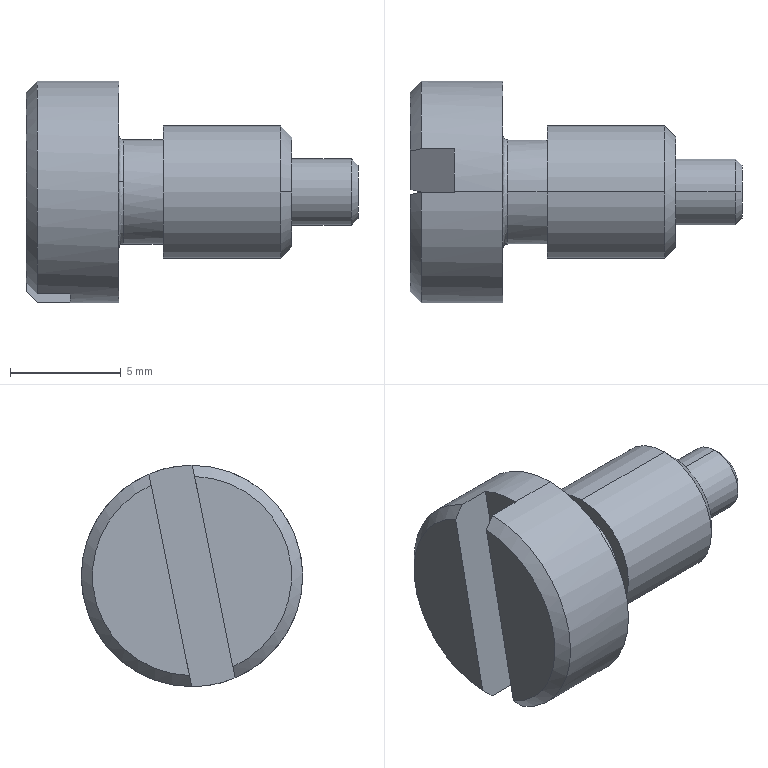Part | SolidWorks | features BaseBody 1 | 1 solid | 25 faces | box 15 x 10 x 10 mm | volume 504.228 mm3 | plane 9 | cylinder 8 | cone 6 | spline 2 | commonest cylinder face diameters 3 x2 4.7 x2 6 x2 10 x2
STEP:
#1=CARTESIAN_POINT('',(-32.901,8.92,2.5));
#2=VERTEX_POINT('',#1);
#3=CARTESIAN_POINT('',(-32.901,8.92,12.5));
#4=VERTEX_POINT('',#3);
#5=CARTESIAN_POINT('',(-32.901,8.92,7.5));
#6=DIRECTION('',(1.,0.,0.));
#7=DIRECTION('',(0.,0.,1.));
#8=AXIS2_PLACEMENT_3D('',#5,#6,#7);
#9=CIRCLE('',#8,5.);
#10=EDGE_CURVE('',#2,#4,#9,.T.);
#11=ORIENTED_EDGE('',*,*,#10,.F.);
#12=CARTESIAN_POINT('',(-35.101,8.92,2.5));
#13=VERTEX_POINT('',#12);
#14=CARTESIAN_POINT('',(-32.901,8.92,2.5));
#15=DIRECTION('',(-1.,0.,0.));
#16=VECTOR('',#15,1000.);
#17=LINE('',#14,#16);
#18=EDGE_CURVE('',#2,#13,#17,.T.);
#19=ORIENTED_EDGE('',*,*,#18,.T.);
#20=CARTESIAN_POINT('',(-35.101,8.937,2.5));
#21=VERTEX_POINT('',#20);
#22=CARTESIAN_POINT('',(-35.101,8.92,7.5));
#23=DIRECTION('',(1.,0.,0.));
#24=DIRECTION('',(0.,0.,1.));
#25=AXIS2_PLACEMENT_3D('',#22,#23,#24);
#26=CIRCLE('',#25,5.);
#27=EDGE_CURVE('',#13,#21,#26,.T.);
#28=ORIENTED_EDGE('',*,*,#27,.T.);
#29=CARTESIAN_POINT('',(-36.601,8.937,2.5));
#30=VERTEX_POINT('',#29);
#31=CARTESIAN_POINT('',(-36.101,8.937,2.5));
#32=DIRECTION('',(-1.,0.,0.));
#33=VECTOR('',#32,1000.);
#34=LINE('',#31,#33);
#35=EDGE_CURVE('',#21,#30,#34,.T.);
#36=ORIENTED_EDGE('',*,*,#35,.T.);
#37=CARTESIAN_POINT('',(-36.601,10.864,12.107));
#38=VERTEX_POINT('',#37);
#39=CARTESIAN_POINT('',(-36.601,8.92,7.5));
#40=DIRECTION('',(1.,0.,0.));
#41=DIRECTION('',(0.,0.,1.));
#42=AXIS2_PLACEMENT_3D('',#39,#40,#41);
#43=CIRCLE('',#42,5.);
#44=EDGE_CURVE('',#30,#38,#43,.T.);
#45=ORIENTED_EDGE('',*,*,#44,.T.);
#46=CARTESIAN_POINT('',(-35.101,10.864,12.107));
#47=VERTEX_POINT('',#46);
#48=CARTESIAN_POINT('',(-36.101,10.864,12.107));
#49=DIRECTION('',(1.,0.,0.));
#50=VECTOR('',#49,1000.);
#51=LINE('',#48,#50);
#52=EDGE_CURVE('',#38,#47,#51,.T.);
#53=ORIENTED_EDGE('',*,*,#52,.T.);
#54=CARTESIAN_POINT('',(-35.101,8.92,12.5));
#55=VERTEX_POINT('',#54);
#56=CARTESIAN_POINT('',(-35.101,8.92,7.5));
#57=DIRECTION('',(1.,0.,0.));
#58=DIRECTION('',(0.,0.,1.));
#59=AXIS2_PLACEMENT_3D('',#56,#57,#58);
#60=CIRCLE('',#59,5.);
#61=EDGE_CURVE('',#47,#55,#60,.T.);
#62=ORIENTED_EDGE('',*,*,#61,.T.);
#63=CARTESIAN_POINT('',(-32.901,8.92,12.5));
#64=DIRECTION('',(-1.,0.,0.));
#65=VECTOR('',#64,1000.);
#66=LINE('',#63,#65);
#67=EDGE_CURVE('',#4,#55,#66,.T.);
#68=ORIENTED_EDGE('',*,*,#67,.F.);
#69=EDGE_LOOP('',(#11,#19,#28,#36,#45,#53,#62,#68));
#70=FACE_OUTER_BOUND('',#69,.T.);
#71=CARTESIAN_POINT('',(-32.901,8.92,7.5));
#72=DIRECTION('',(-1.,0.,0.));
#73=DIRECTION('',(0.,0.,1.));
#74=AXIS2_PLACEMENT_3D('',#71,#72,#73);
#75=CYLINDRICAL_SURFACE('',#74,5.);
#76=ADVANCED_FACE('',(#70),#75,.T.);
#77=CARTESIAN_POINT('',(-30.901,8.92,9.85));
#78=VERTEX_POINT('',#77);
#79=CARTESIAN_POINT('',(-30.901,8.92,5.15));
#80=VERTEX_POINT('',#79);
#81=CARTESIAN_POINT('',(-30.901,8.92,7.5));
#82=DIRECTION('',(-1.,0.,0.));
#83=DIRECTION('',(0.,0.,1.));
#84=AXIS2_PLACEMENT_3D('',#81,#82,#83);
#85=CIRCLE('',#84,2.35);
#86=EDGE_CURVE('',#78,#80,#85,.T.);
#87=ORIENTED_EDGE('',*,*,#86,.T.);
#88=CARTESIAN_POINT('',(-32.701,8.92,5.15));
#89=VERTEX_POINT('',#88);
#90=CARTESIAN_POINT('',(-30.901,8.92,5.15));
#91=DIRECTION('',(-1.,0.,0.));
#92=VECTOR('',#91,1000.);
#93=LINE('',#90,#92);
#94=EDGE_CURVE('',#80,#89,#93,.T.);
#95=ORIENTED_EDGE('',*,*,#94,.T.);
#96=CARTESIAN_POINT('',(-32.701,11.224,7.038));
#97=VERTEX_POINT('',#96);
#98=CARTESIAN_POINT('',(-32.701,8.92,7.5));
#99=DIRECTION('',(1.,0.,0.000000002));
#100=DIRECTION('',(0.,0.9805,-0.1967));
#101=AXIS2_PLACEMENT_3D('',#98,#99,#100);
#102=CIRCLE('',#101,2.35);
#103=EDGE_CURVE('',#89,#97,#102,.T.);
#104=ORIENTED_EDGE('',*,*,#103,.T.);
#105=CARTESIAN_POINT('',(-32.701,8.92,9.85));
#106=VERTEX_POINT('',#105);
#107=CARTESIAN_POINT('',(-32.701,8.92,7.5));
#108=DIRECTION('',(1.,-0.000000001,-0.000000003));
#109=DIRECTION('',(0.,-0.9805,0.1967));
#110=AXIS2_PLACEMENT_3D('',#107,#108,#109);
#111=CIRCLE('',#110,2.35);
#112=EDGE_CURVE('',#97,#106,#111,.T.);
#113=ORIENTED_EDGE('',*,*,#112,.T.);
#114=CARTESIAN_POINT('',(-30.901,8.92,9.85));
#115=DIRECTION('',(-1.,0.,0.));
#116=VECTOR('',#115,1000.);
#117=LINE('',#114,#116);
#118=EDGE_CURVE('',#78,#106,#117,.T.);
#119=ORIENTED_EDGE('',*,*,#118,.F.);
#120=EDGE_LOOP('',(#87,#95,#104,#113,#119));
#121=FACE_OUTER_BOUND('',#120,.T.);
#122=CARTESIAN_POINT('',(-30.901,8.92,7.5));
#123=DIRECTION('',(-1.,0.,0.));
#124=DIRECTION('',(0.,0.,1.));
#125=AXIS2_PLACEMENT_3D('',#122,#123,#124);
#126=CYLINDRICAL_SURFACE('',#125,2.35);
#127=ADVANCED_FACE('',(#121),#126,.T.);
#128=CARTESIAN_POINT('',(-25.601,11.92,7.5));
#129=VERTEX_POINT('',#128);
#130=CARTESIAN_POINT('',(-25.601,8.92,4.5));
#131=VERTEX_POINT('',#130);
#132=CARTESIAN_POINT('',(-25.601,8.92,7.5));
#133=DIRECTION('',(-1.,0.,0.));
#134=DIRECTION('',(0.,0.,1.));
#135=AXIS2_PLACEMENT_3D('',#132,#133,#134);
#136=CIRCLE('',#135,3.);
#137=EDGE_CURVE('',#129,#131,#136,.T.);
#138=ORIENTED_EDGE('',*,*,#137,.T.);
#139=CARTESIAN_POINT('',(-30.901,8.92,4.5));
#140=VERTEX_POINT('',#139);
#141=CARTESIAN_POINT('',(-25.601,8.92,4.5));
#142=DIRECTION('',(-1.,0.,0.));
#143=VECTOR('',#142,1000.);
#144=LINE('',#141,#143);
#145=EDGE_CURVE('',#131,#140,#144,.T.);
#146=ORIENTED_EDGE('',*,*,#145,.T.);
#147=CARTESIAN_POINT('',(-30.901,8.92,10.5));
#148=VERTEX_POINT('',#147);
#149=CARTESIAN_POINT('',(-30.901,8.92,7.5));
#150=DIRECTION('',(1.,0.,0.));
#151=DIRECTION('',(0.,0.,1.));
#152=AXIS2_PLACEMENT_3D('',#149,#150,#151);
#153=CIRCLE('',#152,3.);
#154=EDGE_CURVE('',#140,#148,#153,.T.);
#155=ORIENTED_EDGE('',*,*,#154,.T.);
#156=CARTESIAN_POINT('',(-25.601,8.92,10.5));
#157=VERTEX_POINT('',#156);
#158=CARTESIAN_POINT('',(-25.601,8.92,10.5));
#159=DIRECTION('',(-1.,0.,0.));
#160=VECTOR('',#159,1000.);
#161=LINE('',#158,#160);
#162=EDGE_CURVE('',#157,#148,#161,.T.);
#163=ORIENTED_EDGE('',*,*,#162,.F.);
#164=CARTESIAN_POINT('',(-25.601,8.92,7.5));
#165=DIRECTION('',(-1.,0.,0.));
#166=DIRECTION('',(0.,0.,1.));
#167=AXIS2_PLACEMENT_3D('',#164,#165,#166);
#168=CIRCLE('',#167,3.);
#169=EDGE_CURVE('',#157,#129,#168,.T.);
#170=ORIENTED_EDGE('',*,*,#169,.T.);
#171=EDGE_LOOP('',(#138,#146,#155,#163,#170));
#172=FACE_OUTER_BOUND('',#171,.T.);
#173=CARTESIAN_POINT('',(-25.601,8.92,7.5));
#174=DIRECTION('',(-1.,0.,0.));
#175=DIRECTION('',(0.,0.,1.));
#176=AXIS2_PLACEMENT_3D('',#173,#174,#175);
#177=CYLINDRICAL_SURFACE('',#176,3.);
#178=ADVANCED_FACE('',(#172),#177,.T.);
#179=CARTESIAN_POINT('',(-25.101,6.42,7.5));
#180=VERTEX_POINT('',#179);
#181=CARTESIAN_POINT('',(-25.101,11.42,7.5));
#182=VERTEX_POINT('',#181);
#183=CARTESIAN_POINT('',(-25.101,8.92,7.5));
#184=DIRECTION('',(-1.,0.,0.));
#185=DIRECTION('',(0.,-1.,0.));
#186=AXIS2_PLACEMENT_3D('',#183,#184,#185);
#187=CIRCLE('',#186,2.5);
#188=EDGE_CURVE('',#180,#182,#187,.T.);
#189=ORIENTED_EDGE('',*,*,#188,.T.);
#190=CARTESIAN_POINT('',(-25.601,11.92,7.5));
#191=DIRECTION('',(-0.7071,0.7071,0.));
#192=VECTOR('',#191,1000.);
#193=LINE('',#190,#192);
#194=EDGE_CURVE('',#182,#129,#193,.T.);
#195=ORIENTED_EDGE('',*,*,#194,.T.);
#196=ORIENTED_EDGE('',*,*,#169,.F.);
#197=CARTESIAN_POINT('',(-25.601,5.92,7.5));
#198=VERTEX_POINT('',#197);
#199=CARTESIAN_POINT('',(-25.601,8.92,7.5));
#200=DIRECTION('',(-1.,0.,0.));
#201=DIRECTION('',(0.,0.,1.));
#202=AXIS2_PLACEMENT_3D('',#199,#200,#201);
#203=CIRCLE('',#202,3.);
#204=EDGE_CURVE('',#198,#157,#203,.T.);
#205=ORIENTED_EDGE('',*,*,#204,.F.);
#206=CARTESIAN_POINT('',(-25.601,5.92,7.5));
#207=DIRECTION('',(-0.7071,-0.7071,0.));
#208=VECTOR('',#207,1000.);
#209=LINE('',#206,#208);
#210=EDGE_CURVE('',#180,#198,#209,.T.);
#211=ORIENTED_EDGE('',*,*,#210,.F.);
#212=EDGE_LOOP('',(#189,#195,#196,#205,#211));
#213=FACE_OUTER_BOUND('',#212,.T.);
#214=CARTESIAN_POINT('',(-25.601,8.92,7.5));
#215=DIRECTION('',(-1.,0.,0.));
#216=DIRECTION('',(0.,-1.,0.));
#217=AXIS2_PLACEMENT_3D('',#214,#215,#216);
#218=CONICAL_SURFACE('',#217,3.,0.7854);
#219=ADVANCED_FACE('',(#213),#218,.T.);
#220=CARTESIAN_POINT('',(-22.401,8.92,9.));
#221=VERTEX_POINT('',#220);
#222=CARTESIAN_POINT('',(-22.401,8.92,6.));
#223=VERTEX_POINT('',#222);
#224=CARTESIAN_POINT('',(-22.401,8.92,7.5));
#225=DIRECTION('',(-1.,0.,0.));
#226=DIRECTION('',(0.,0.,1.));
#227=AXIS2_PLACEMENT_3D('',#224,#225,#226);
#228=CIRCLE('',#227,1.5);
#229=EDGE_CURVE('',#221,#223,#228,.T.);
#230=ORIENTED_EDGE('',*,*,#229,.T.);
#231=CARTESIAN_POINT('',(-25.101,8.92,6.));
#232=VERTEX_POINT('',#231);
#233=CARTESIAN_POINT('',(-22.401,8.92,6.));
#234=DIRECTION('',(-1.,0.,0.));
#235=VECTOR('',#234,1000.);
#236=LINE('',#233,#235);
#237=EDGE_CURVE('',#223,#232,#236,.T.);
#238=ORIENTED_EDGE('',*,*,#237,.T.);
#239=CARTESIAN_POINT('',(-25.101,8.92,9.));
#240=VERTEX_POINT('',#239);
#241=CARTESIAN_POINT('',(-25.101,8.92,7.5));
#242=DIRECTION('',(-1.,0.,0.));
#243=DIRECTION('',(0.,0.,1.));
#244=AXIS2_PLACEMENT_3D('',#241,#242,#243);
#245=CIRCLE('',#244,1.5);
#246=EDGE_CURVE('',#240,#232,#245,.T.);
#247=ORIENTED_EDGE('',*,*,#246,.F.);
#248=CARTESIAN_POINT('',(-22.401,8.92,9.));
#249=DIRECTION('',(-1.,0.,0.));
#250=VECTOR('',#249,1000.);
#251=LINE('',#248,#250);
#252=EDGE_CURVE('',#221,#240,#251,.T.);
#253=ORIENTED_EDGE('',*,*,#252,.F.);
#254=EDGE_LOOP('',(#230,#238,#247,#253));
#255=FACE_OUTER_BOUND('',#254,.T.);
#256=CARTESIAN_POINT('',(-22.401,8.92,7.5));
#257=DIRECTION('',(-1.,0.,0.));
#258=DIRECTION('',(0.,0.,1.));
#259=AXIS2_PLACEMENT_3D('',#256,#257,#258);
#260=CYLINDRICAL_SURFACE('',#259,1.5);
#261=ADVANCED_FACE('',(#255),#260,.T.);
#262=CARTESIAN_POINT('',(-22.101,8.92,8.7));
#263=VERTEX_POINT('',#262);
#264=CARTESIAN_POINT('',(-22.101,8.92,6.3));
#265=VERTEX_POINT('',#264);
#266=CARTESIAN_POINT('',(-22.101,8.92,7.5));
#267=DIRECTION('',(-1.,0.,0.));
#268=DIRECTION('',(0.,0.,1.));
#269=AXIS2_PLACEMENT_3D('',#266,#267,#268);
#270=CIRCLE('',#269,1.2);
#271=EDGE_CURVE('',#263,#265,#270,.T.);
#272=ORIENTED_EDGE('',*,*,#271,.T.);
#273=CARTESIAN_POINT('',(-22.401,8.92,6.));
#274=DIRECTION('',(-0.7071,0.,-0.7071));
#275=VECTOR('',#274,1000.);
#276=LINE('',#273,#275);
#277=EDGE_CURVE('',#265,#223,#276,.T.);
#278=ORIENTED_EDGE('',*,*,#277,.T.);
#279=ORIENTED_EDGE('',*,*,#229,.F.);
#280=CARTESIAN_POINT('',(-22.401,8.92,9.));
#281=DIRECTION('',(-0.7071,0.,0.7071));
#282=VECTOR('',#281,1000.);
#283=LINE('',#280,#282);
#284=EDGE_CURVE('',#263,#221,#283,.T.);
#285=ORIENTED_EDGE('',*,*,#284,.F.);
#286=EDGE_LOOP('',(#272,#278,#279,#285));
#287=FACE_OUTER_BOUND('',#286,.T.);
#288=CARTESIAN_POINT('',(-22.401,8.92,7.5));
#289=DIRECTION('',(-1.,0.,0.));
#290=DIRECTION('',(0.,0.,1.));
#291=AXIS2_PLACEMENT_3D('',#288,#289,#290);
#292=CONICAL_SURFACE('',#291,1.5,0.7854);
#293=ADVANCED_FACE('',(#287),#292,.T.);
#294=CARTESIAN_POINT('',(-32.901,6.42,8.002));
#295=VERTEX_POINT('',#294);
#296=CARTESIAN_POINT('',(-32.901,11.42,6.998));
#297=VERTEX_POINT('',#296);
#298=CARTESIAN_POINT('',(-32.901,6.42,8.002));
#299=CARTESIAN_POINT('',(-32.901,6.452,8.161));
#300=CARTESIAN_POINT('',(-32.901,6.52,8.39));
#301=CARTESIAN_POINT('',(-32.901,6.638,8.643));
#302=CARTESIAN_POINT('',(-32.901,6.706,8.766));
#303=CARTESIAN_POINT('',(-32.901,6.737,8.818));
#304=CARTESIAN_POINT('',(-32.901,6.758,8.853));
#305=CARTESIAN_POINT('',(-32.901,6.768,8.868));
#306=CARTESIAN_POINT('',(-32.901,6.971,9.182));
#307=CARTESIAN_POINT('',(-32.901,7.214,9.428));
#308=CARTESIAN_POINT('',(-32.901,7.653,9.72));
#309=CARTESIAN_POINT('',(-32.901,7.883,9.842));
#310=CARTESIAN_POINT('',(-32.901,8.168,9.94));
#311=CARTESIAN_POINT('',(-32.901,8.316,9.978));
#312=CARTESIAN_POINT('',(-32.901,8.38,9.992));
#313=CARTESIAN_POINT('',(-32.901,8.423,10.001));
#314=CARTESIAN_POINT('',(-32.901,8.446,10.006));
#315=CARTESIAN_POINT('',(-32.901,8.785,10.067));
#316=CARTESIAN_POINT('',(-32.901,9.104,10.064));
#317=CARTESIAN_POINT('',(-32.901,9.58,9.968));
#318=CARTESIAN_POINT('',(-32.901,9.81,9.899));
#319=CARTESIAN_POINT('',(-32.901,10.063,9.782));
#320=CARTESIAN_POINT('',(-32.901,10.186,9.714));
#321=CARTESIAN_POINT('',(-32.901,10.238,9.683));
#322=CARTESIAN_POINT('',(-32.901,10.272,9.662));
#323=CARTESIAN_POINT('',(-32.901,10.288,9.652));
#324=CARTESIAN_POINT('',(-32.901,10.602,9.449));
#325=CARTESIAN_POINT('',(-32.901,10.847,9.206));
#326=CARTESIAN_POINT('',(-32.901,11.14,8.767));
#327=CARTESIAN_POINT('',(-32.901,11.261,8.537));
#328=CARTESIAN_POINT('',(-32.901,11.36,8.251));
#329=CARTESIAN_POINT('',(-32.901,11.398,8.104));
#330=CARTESIAN_POINT('',(-32.901,11.412,8.04));
#331=CARTESIAN_POINT('',(-32.901,11.421,7.997));
#332=CARTESIAN_POINT('',(-32.901,11.425,7.974));
#333=CARTESIAN_POINT('',(-32.901,11.487,7.635));
#334=CARTESIAN_POINT('',(-32.901,11.484,7.316));
#335=CARTESIAN_POINT('',(-32.901,11.42,6.998));
#336=B_SPLINE_CURVE_WITH_KNOTS('',3,(#298,#299,#300,#301,#302,#303,#304,#305,#306,#307,#308,#309,#310,#311,#312,#313,#314,#315,#316,#317,#318,#319,#320,#321,#322,#323,#324,#325,#326,#327,#328,#329,#330,#331,#332,#333,#334,#335),.UNSPECIFIED.,.F.,.F.,(4,1,1,1,2,2,2,1,1,1,2,2,2,1,1,1,2,2,2,1,1,1,2,2,4),(0.,0.0625,0.09375,0.1094,0.1172,0.125,0.25,0.3125,0.3438,0.3594,0.3672,0.375,0.5,0.5625,0.5938,0.6094,0.6172,0.625,0.75,0.8125,0.8437,0.8594,0.8672,0.875,1.),.UNSPECIFIED.);
#337=EDGE_CURVE('',#295,#297,#336,.T.);
#338=ORIENTED_EDGE('',*,*,#337,.T.);
#339=CARTESIAN_POINT('',(-32.901,11.42,6.998));
#340=CARTESIAN_POINT('',(-32.901,11.387,6.834));
#341=CARTESIAN_POINT('',(-32.901,11.315,6.597));
#342=CARTESIAN_POINT('',(-32.901,11.209,6.373));
#343=CARTESIAN_POINT('',(-32.901,11.131,6.227));
#344=CARTESIAN_POINT('',(-32.901,11.09,6.158));
#345=CARTESIAN_POINT('',(-32.901,10.946,5.943));
#346=CARTESIAN_POINT('',(-32.901,10.785,5.746));
#347=CARTESIAN_POINT('',(-32.901,10.565,5.548));
#348=CARTESIAN_POINT('',(-32.901,10.464,5.47));
#349=CARTESIAN_POINT('',(-32.901,10.395,5.419));
#350=CARTESIAN_POINT('',(-32.901,10.358,5.394));
#351=CARTESIAN_POINT('',(-32.901,10.185,5.28));
#352=CARTESIAN_POINT('',(-32.901,9.969,5.166));
#353=CARTESIAN_POINT('',(-32.901,9.702,5.07));
#354=CARTESIAN_POINT('',(-32.901,9.583,5.037));
#355=CARTESIAN_POINT('',(-32.901,9.504,5.017));
#356=CARTESIAN_POINT('',(-32.901,9.465,5.009));
#357=CARTESIAN_POINT('',(-32.901,9.088,4.933));
#358=CARTESIAN_POINT('',(-32.901,8.753,4.933));
#359=CARTESIAN_POINT('',(-32.901,8.251,5.033));
#360=CARTESIAN_POINT('',(-32.901,8.01,5.107));
#361=CARTESIAN_POINT('',(-32.901,7.745,5.234));
#362=CARTESIAN_POINT('',(-32.901,7.635,5.297));
#363=CARTESIAN_POINT('',(-32.901,7.562,5.341));
#364=CARTESIAN_POINT('',(-32.901,7.525,5.365));
#365=CARTESIAN_POINT('',(-32.901,7.354,5.48));
#366=CARTESIAN_POINT('',(-32.901,7.166,5.636));
#367=CARTESIAN_POINT('',(-32.901,6.975,5.847));
#368=CARTESIAN_POINT('',(-32.901,6.9,5.943));
#369=CARTESIAN_POINT('',(-32.901,6.851,6.009));
#370=CARTESIAN_POINT('',(-32.901,6.828,6.041));
#371=CARTESIAN_POINT('',(-32.901,6.708,6.22));
#372=CARTESIAN_POINT('',(-32.901,6.587,6.444));
#373=CARTESIAN_POINT('',(-32.901,6.488,6.723));
#374=CARTESIAN_POINT('',(-32.901,6.454,6.847));
#375=CARTESIAN_POINT('',(-32.901,6.434,6.93));
#376=CARTESIAN_POINT('',(-32.901,6.425,6.973));
#377=CARTESIAN_POINT('',(-32.901,6.353,7.343));
#378=CARTESIAN_POINT('',(-32.901,6.354,7.672));
#379=CARTESIAN_POINT('',(-32.901,6.42,8.002));
#380=B_SPLINE_CURVE_WITH_KNOTS('',3,(#339,#340,#341,#342,#343,#344,#345,#346,#347,#348,#349,#350,#351,#352,#353,#354,#355,#356,#357,#358,#359,#360,#361,#362,#363,#364,#365,#366,#367,#368,#369,#370,#371,#372,#373,#374,#375,#376,#377,#378,#379),.UNSPECIFIED.,.F.,.F.,(4,1,2,2,1,1,2,2,1,1,2,2,2,1,1,2,2,1,1,2,2,1,1,2,2,4),(0.,0.0625,0.09375,0.125,0.1875,0.2187,0.2344,0.25,0.3125,0.3437,0.3594,0.375,0.5,0.5625,0.5937,0.6094,0.625,0.6875,0.7187,0.7344,0.75,0.8125,0.8437,0.8594,0.875,1.),.UNSPECIFIED.);
#381=EDGE_CURVE('',#297,#295,#380,.T.);
#382=ORIENTED_EDGE('',*,*,#381,.T.);
#383=EDGE_LOOP('',(#338,#382));
#384=FACE_BOUND('',#383,.T.);
#385=CARTESIAN_POINT('',(-32.901,8.92,7.5));
#386=DIRECTION('',(1.,0.,0.));
#387=DIRECTION('',(0.,0.,1.));
#388=AXIS2_PLACEMENT_3D('',#385,#386,#387);
#389=CIRCLE('',#388,5.);
#390=EDGE_CURVE('',#4,#2,#389,.T.);
#391=ORIENTED_EDGE('',*,*,#390,.T.);
#392=ORIENTED_EDGE('',*,*,#10,.T.);
#393=EDGE_LOOP('',(#391,#392));
#394=FACE_OUTER_BOUND('',#393,.T.);
#395=CARTESIAN_POINT('',(-32.901,8.92,7.5));
#396=DIRECTION('',(1.,0.,0.));
#397=DIRECTION('',(0.,0.,-1.));
#398=AXIS2_PLACEMENT_3D('',#395,#396,#397);
#399=PLANE('',#398);
#400=ADVANCED_FACE('',(#384,#394),#399,.T.);
#401=CARTESIAN_POINT('',(-32.701,6.616,7.962));
#402=VERTEX_POINT('',#401);
#403=CARTESIAN_POINT('',(-32.701,8.92,7.5));
#404=DIRECTION('',(1.,0.,0.000000002));
#405=DIRECTION('',(0.,0.9805,-0.1967));
#406=AXIS2_PLACEMENT_3D('',#403,#404,#405);
#407=CIRCLE('',#406,2.35);
#408=EDGE_CURVE('',#402,#89,#407,.T.);
#409=ORIENTED_EDGE('',*,*,#408,.F.);
#410=CARTESIAN_POINT('',(-32.701,6.42,8.002));
#411=DIRECTION('',(0.000000002,-0.1967,-0.9805));
#412=DIRECTION('',(0.,-0.9805,0.1967));
#413=AXIS2_PLACEMENT_3D('',#410,#411,#412);
#414=CIRCLE('',#413,0.2);
#415=EDGE_CURVE('',#295,#402,#414,.T.);
#416=ORIENTED_EDGE('',*,*,#415,.F.);
#417=ORIENTED_EDGE('',*,*,#381,.F.);
#418=CARTESIAN_POINT('',(-32.701,11.42,6.998));
#419=DIRECTION('',(-0.000000003,-0.1967,-0.9805));
#420=DIRECTION('',(0.,0.9805,-0.1967));
#421=AXIS2_PLACEMENT_3D('',#418,#419,#420);
#422=CIRCLE('',#421,0.2);
#423=EDGE_CURVE('',#97,#297,#422,.T.);
#424=ORIENTED_EDGE('',*,*,#423,.F.);
#425=ORIENTED_EDGE('',*,*,#103,.F.);
#426=EDGE_LOOP('',(#409,#416,#417,#424,#425));
#427=FACE_OUTER_BOUND('',#426,.T.);
#428=CARTESIAN_POINT('',(-32.701,11.224,7.038));
#429=CARTESIAN_POINT('',(-32.701,10.953,5.688));
#430=CARTESIAN_POINT('',(-32.701,9.807,4.925));
#431=CARTESIAN_POINT('',(-32.701,8.458,5.196));
#432=CARTESIAN_POINT('',(-32.701,7.108,5.467));
#433=CARTESIAN_POINT('',(-32.701,6.345,6.613));
#434=CARTESIAN_POINT('',(-32.701,6.616,7.962));
#435=CARTESIAN_POINT('',(-32.818,11.224,7.038));
#436=CARTESIAN_POINT('',(-32.818,10.953,5.688));
#437=CARTESIAN_POINT('',(-32.818,9.807,4.925));
#438=CARTESIAN_POINT('',(-32.818,8.458,5.196));
#439=CARTESIAN_POINT('',(-32.818,7.108,5.467));
#440=CARTESIAN_POINT('',(-32.818,6.345,6.613));
#441=CARTESIAN_POINT('',(-32.818,6.616,7.962));
#442=CARTESIAN_POINT('',(-32.901,11.305,7.021));
#443=CARTESIAN_POINT('',(-32.901,11.025,5.624));
#444=CARTESIAN_POINT('',(-32.901,9.838,4.834));
#445=CARTESIAN_POINT('',(-32.901,8.441,5.115));
#446=CARTESIAN_POINT('',(-32.901,7.044,5.395));
#447=CARTESIAN_POINT('',(-32.901,6.254,6.581));
#448=CARTESIAN_POINT('',(-32.901,6.535,7.979));
#449=CARTESIAN_POINT('',(-32.901,11.42,6.998));
#450=CARTESIAN_POINT('',(-32.901,11.126,5.534));
#451=CARTESIAN_POINT('',(-32.901,9.883,4.706));
#452=CARTESIAN_POINT('',(-32.901,8.418,5.));
#453=CARTESIAN_POINT('',(-32.901,6.954,5.294));
#454=CARTESIAN_POINT('',(-32.901,6.126,6.537));
#455=CARTESIAN_POINT('',(-32.901,6.42,8.002));
#456=(BOUNDED_SURFACE()B_SPLINE_SURFACE(3,3,((#428,#429,#430,#431,#432,#433,#434),(#435,#436,#437,#438,#439,#440,#441),(#442,#443,#444,#445,#446,#447,#448),(#449,#450,#451,#452,#453,#454,#455)),.UNSPECIFIED.,.F.,.F.,.T.)B_SPLINE_SURFACE_WITH_KNOTS((4,4),(4,3,4),(0.,1.),(0.,0.5,1.),.UNSPECIFIED.)GEOMETRIC_REPRESENTATION_ITEM()RATIONAL_B_SPLINE_SURFACE(((1.,0.8047,0.8047,1.,0.8047,0.8047,1.),(0.8047,0.6476,0.6476,0.8047,0.6476,0.6476,0.8047),(0.8047,0.6476,0.6476,0.8047,0.6476,0.6476,0.8047),(1.,0.8047,0.8047,1.,0.8047,0.8047,1.)))REPRESENTATION_ITEM('')SURFACE());
#457=ADVANCED_FACE('',(#427),#456,.F.);
#458=ORIENTED_EDGE('',*,*,#337,.F.);
#459=ORIENTED_EDGE('',*,*,#415,.T.);
#460=CARTESIAN_POINT('',(-32.701,8.92,7.5));
#461=DIRECTION('',(1.,-0.000000001,-0.000000003));
#462=DIRECTION('',(0.,-0.9805,0.1967));
#463=AXIS2_PLACEMENT_3D('',#460,#461,#462);
#464=CIRCLE('',#463,2.35);
#465=EDGE_CURVE('',#106,#402,#464,.T.);
#466=ORIENTED_EDGE('',*,*,#465,.F.);
#467=ORIENTED_EDGE('',*,*,#112,.F.);
#468=ORIENTED_EDGE('',*,*,#423,.T.);
#469=EDGE_LOOP('',(#458,#459,#466,#467,#468));
#470=FACE_OUTER_BOUND('',#469,.T.);
#471=CARTESIAN_POINT('',(-32.701,6.616,7.962));
#472=CARTESIAN_POINT('',(-32.701,6.887,9.312));
#473=CARTESIAN_POINT('',(-32.701,8.032,10.075));
#474=CARTESIAN_POINT('',(-32.701,9.382,9.804));
#475=CARTESIAN_POINT('',(-32.701,10.732,9.533));
#476=CARTESIAN_POINT('',(-32.701,11.495,8.387));
#477=CARTESIAN_POINT('',(-32.701,11.224,7.038));
#478=CARTESIAN_POINT('',(-32.818,6.616,7.962));
#479=CARTESIAN_POINT('',(-32.818,6.887,9.312));
#480=CARTESIAN_POINT('',(-32.818,8.032,10.075));
#481=CARTESIAN_POINT('',(-32.818,9.382,9.804));
#482=CARTESIAN_POINT('',(-32.818,10.732,9.533));
#483=CARTESIAN_POINT('',(-32.818,11.495,8.387));
#484=CARTESIAN_POINT('',(-32.818,11.224,7.038));
#485=CARTESIAN_POINT('',(-32.901,6.535,7.979));
#486=CARTESIAN_POINT('',(-32.901,6.815,9.376));
#487=CARTESIAN_POINT('',(-32.901,8.001,10.166));
#488=CARTESIAN_POINT('',(-32.901,9.398,9.885));
#489=CARTESIAN_POINT('',(-32.901,10.796,9.605));
#490=CARTESIAN_POINT('',(-32.901,11.585,8.419));
#491=CARTESIAN_POINT('',(-32.901,11.305,7.021));
#492=CARTESIAN_POINT('',(-32.901,6.42,8.002));
#493=CARTESIAN_POINT('',(-32.901,6.713,9.466));
#494=CARTESIAN_POINT('',(-32.901,7.957,10.294));
#495=CARTESIAN_POINT('',(-32.901,9.421,10.));
#496=CARTESIAN_POINT('',(-32.901,10.886,9.706));
#497=CARTESIAN_POINT('',(-32.901,11.714,8.463));
#498=CARTESIAN_POINT('',(-32.901,11.42,6.998));
#499=(BOUNDED_SURFACE()B_SPLINE_SURFACE(3,3,((#471,#472,#473,#474,#475,#476,#477),(#478,#479,#480,#481,#482,#483,#484),(#485,#486,#487,#488,#489,#490,#491),(#492,#493,#494,#495,#496,#497,#498)),.UNSPECIFIED.,.F.,.F.,.T.)B_SPLINE_SURFACE_WITH_KNOTS((4,4),(4,3,4),(0.,1.),(0.,0.5,1.),.UNSPECIFIED.)GEOMETRIC_REPRESENTATION_ITEM()RATIONAL_B_SPLINE_SURFACE(((1.,0.8047,0.8047,1.,0.8047,0.8047,1.),(0.8047,0.6476,0.6476,0.8047,0.6476,0.6476,0.8047),(0.8047,0.6476,0.6476,0.8047,0.6476,0.6476,0.8047),(1.,0.8047,0.8047,1.,0.8047,0.8047,1.)))REPRESENTATION_ITEM('')SURFACE());
#500=ADVANCED_FACE('',(#470),#499,.F.);
#501=ORIENTED_EDGE('',*,*,#18,.F.);
#502=ORIENTED_EDGE('',*,*,#390,.F.);
#503=ORIENTED_EDGE('',*,*,#67,.T.);
#504=CARTESIAN_POINT('',(-35.101,8.903,12.5));
#505=VERTEX_POINT('',#504);
#506=CARTESIAN_POINT('',(-35.101,8.92,7.5));
#507=DIRECTION('',(1.,0.,0.));
#508=DIRECTION('',(0.,0.,1.));
#509=AXIS2_PLACEMENT_3D('',#506,#507,#508);
#510=CIRCLE('',#509,5.);
#511=EDGE_CURVE('',#55,#505,#510,.T.);
#512=ORIENTED_EDGE('',*,*,#511,.T.);
#513=CARTESIAN_POINT('',(-36.601,8.903,12.5));
#514=VERTEX_POINT('',#513);
#515=CARTESIAN_POINT('',(-36.101,8.903,12.5));
#516=DIRECTION('',(1.,0.,0.));
#517=VECTOR('',#516,1000.);
#518=LINE('',#515,#517);
#519=EDGE_CURVE('',#514,#505,#518,.T.);
#520=ORIENTED_EDGE('',*,*,#519,.F.);
#521=CARTESIAN_POINT('',(-36.601,6.976,2.893));
#522=VERTEX_POINT('',#521);
#523=CARTESIAN_POINT('',(-36.601,8.92,7.5));
#524=DIRECTION('',(1.,0.,0.));
#525=DIRECTION('',(0.,0.,1.));
#526=AXIS2_PLACEMENT_3D('',#523,#524,#525);
#527=CIRCLE('',#526,5.);
#528=EDGE_CURVE('',#514,#522,#527,.T.);
#529=ORIENTED_EDGE('',*,*,#528,.T.);
#530=CARTESIAN_POINT('',(-35.101,6.976,2.893));
#531=VERTEX_POINT('',#530);
#532=CARTESIAN_POINT('',(-36.101,6.976,2.893));
#533=DIRECTION('',(-1.,0.,0.));
#534=VECTOR('',#533,1000.);
#535=LINE('',#532,#534);
#536=EDGE_CURVE('',#531,#522,#535,.T.);
#537=ORIENTED_EDGE('',*,*,#536,.F.);
#538=CARTESIAN_POINT('',(-35.101,8.92,7.5));
#539=DIRECTION('',(1.,0.,0.));
#540=DIRECTION('',(0.,0.,1.));
#541=AXIS2_PLACEMENT_3D('',#538,#539,#540);
#542=CIRCLE('',#541,5.);
#543=EDGE_CURVE('',#531,#13,#542,.T.);
#544=ORIENTED_EDGE('',*,*,#543,.T.);
#545=EDGE_LOOP('',(#501,#502,#503,#512,#520,#529,#537,#544));
#546=FACE_OUTER_BOUND('',#545,.T.);
#547=CARTESIAN_POINT('',(-32.901,8.92,7.5));
#548=DIRECTION('',(-1.,0.,0.));
#549=DIRECTION('',(0.,0.,1.));
#550=AXIS2_PLACEMENT_3D('',#547,#548,#549);
#551=CYLINDRICAL_SURFACE('',#550,5.);
#552=ADVANCED_FACE('',(#546),#551,.T.);
#553=ORIENTED_EDGE('',*,*,#94,.F.);
#554=CARTESIAN_POINT('',(-30.901,8.92,7.5));
#555=DIRECTION('',(-1.,0.,0.));
#556=DIRECTION('',(0.,0.,1.));
#557=AXIS2_PLACEMENT_3D('',#554,#555,#556);
#558=CIRCLE('',#557,2.35);
#559=EDGE_CURVE('',#80,#78,#558,.T.);
#560=ORIENTED_EDGE('',*,*,#559,.T.);
#561=ORIENTED_EDGE('',*,*,#118,.T.);
#562=ORIENTED_EDGE('',*,*,#465,.T.);
#563=ORIENTED_EDGE('',*,*,#408,.T.);
#564=EDGE_LOOP('',(#553,#560,#561,#562,#563));
#565=FACE_OUTER_BOUND('',#564,.T.);
#566=CARTESIAN_POINT('',(-30.901,8.92,7.5));
#567=DIRECTION('',(-1.,0.,0.));
#568=DIRECTION('',(0.,0.,1.));
#569=AXIS2_PLACEMENT_3D('',#566,#567,#568);
#570=CYLINDRICAL_SURFACE('',#569,2.35);
#571=ADVANCED_FACE('',(#565),#570,.T.);
#572=ORIENTED_EDGE('',*,*,#44,.F.);
#573=CARTESIAN_POINT('',(-37.101,9.037,3.002));
#574=VERTEX_POINT('',#573);
#575=CARTESIAN_POINT('',(-36.601,8.937,2.5));
#576=CARTESIAN_POINT('',(-36.768,8.97,2.667));
#577=CARTESIAN_POINT('',(-36.935,9.004,2.834));
#578=CARTESIAN_POINT('',(-37.101,9.037,3.002));
#579=B_SPLINE_CURVE_WITH_KNOTS('',3,(#575,#576,#577,#578),.UNSPECIFIED.,.F.,.F.,(4,4),(0.,0.0007153),.UNSPECIFIED.);
#580=EDGE_CURVE('',#30,#574,#579,.T.);
#581=ORIENTED_EDGE('',*,*,#580,.T.);
#582=CARTESIAN_POINT('',(-37.101,10.763,11.605));
#583=VERTEX_POINT('',#582);
#584=CARTESIAN_POINT('',(-37.101,8.92,7.5));
#585=DIRECTION('',(1.,0.,0.));
#586=DIRECTION('',(0.,0.,-1.));
#587=AXIS2_PLACEMENT_3D('',#584,#585,#586);
#588=CIRCLE('',#587,4.5);
#589=EDGE_CURVE('',#574,#583,#588,.T.);
#590=ORIENTED_EDGE('',*,*,#589,.T.);
#591=CARTESIAN_POINT('',(-37.101,10.763,11.605));
#592=CARTESIAN_POINT('',(-36.935,10.797,11.772));
#593=CARTESIAN_POINT('',(-36.768,10.83,11.94));
#594=CARTESIAN_POINT('',(-36.601,10.864,12.107));
#595=B_SPLINE_CURVE_WITH_KNOTS('',3,(#591,#592,#593,#594),.UNSPECIFIED.,.F.,.F.,(4,4),(0.,0.0007153),.UNSPECIFIED.);
#596=EDGE_CURVE('',#583,#38,#595,.T.);
#597=ORIENTED_EDGE('',*,*,#596,.T.);
#598=EDGE_LOOP('',(#572,#581,#590,#597));
#599=FACE_OUTER_BOUND('',#598,.T.);
#600=CARTESIAN_POINT('',(-36.601,8.92,7.5));
#601=DIRECTION('',(1.,0.,0.));
#602=DIRECTION('',(0.,0.,-1.));
#603=AXIS2_PLACEMENT_3D('',#600,#601,#602);
#604=CONICAL_SURFACE('',#603,5.,0.7854);
#605=ADVANCED_FACE('',(#599),#604,.T.);
#606=ORIENTED_EDGE('',*,*,#61,.F.);
#607=CARTESIAN_POINT('',(-35.101,8.937,2.5));
#608=DIRECTION('',(0.,0.1967,0.9805));
#609=VECTOR('',#608,1000.);
#610=LINE('',#607,#609);
#611=EDGE_CURVE('',#21,#47,#610,.T.);
#612=ORIENTED_EDGE('',*,*,#611,.F.);
#613=ORIENTED_EDGE('',*,*,#27,.F.);
#614=ORIENTED_EDGE('',*,*,#543,.F.);
#615=CARTESIAN_POINT('',(-35.101,8.903,12.5));
#616=DIRECTION('',(0.,-0.1967,-0.9805));
#617=VECTOR('',#616,1000.);
#618=LINE('',#615,#617);
#619=EDGE_CURVE('',#505,#531,#618,.T.);
#620=ORIENTED_EDGE('',*,*,#619,.F.);
#621=ORIENTED_EDGE('',*,*,#511,.F.);
#622=EDGE_LOOP('',(#606,#612,#613,#614,#620,#621));
#623=FACE_OUTER_BOUND('',#622,.T.);
#624=CARTESIAN_POINT('',(-35.101,8.92,7.5));
#625=DIRECTION('',(1.,0.,0.));
#626=DIRECTION('',(0.,0.,-1.));
#627=AXIS2_PLACEMENT_3D('',#624,#625,#626);
#628=PLANE('',#627);
#629=ADVANCED_FACE('',(#623),#628,.F.);
#630=CARTESIAN_POINT('',(-37.101,8.802,11.998));
#631=VERTEX_POINT('',#630);
#632=CARTESIAN_POINT('',(-37.101,7.076,3.395));
#633=VERTEX_POINT('',#632);
#634=CARTESIAN_POINT('',(-37.101,8.92,7.5));
#635=DIRECTION('',(1.,0.,0.));
#636=DIRECTION('',(0.,0.,-1.));
#637=AXIS2_PLACEMENT_3D('',#634,#635,#636);
#638=CIRCLE('',#637,4.5);
#639=EDGE_CURVE('',#631,#633,#638,.T.);
#640=ORIENTED_EDGE('',*,*,#639,.T.);
#641=CARTESIAN_POINT('',(-37.101,7.076,3.395));
#642=CARTESIAN_POINT('',(-36.935,7.043,3.228));
#643=CARTESIAN_POINT('',(-36.768,7.009,3.06));
#644=CARTESIAN_POINT('',(-36.601,6.976,2.893));
#645=B_SPLINE_CURVE_WITH_KNOTS('',3,(#641,#642,#643,#644),.UNSPECIFIED.,.F.,.F.,(4,4),(0.,0.0007153),.UNSPECIFIED.);
#646=EDGE_CURVE('',#633,#522,#645,.T.);
#647=ORIENTED_EDGE('',*,*,#646,.T.);
#648=ORIENTED_EDGE('',*,*,#528,.F.);
#649=CARTESIAN_POINT('',(-36.601,8.903,12.5));
#650=CARTESIAN_POINT('',(-36.768,8.87,12.333));
#651=CARTESIAN_POINT('',(-36.935,8.836,12.166));
#652=CARTESIAN_POINT('',(-37.101,8.802,11.998));
#653=B_SPLINE_CURVE_WITH_KNOTS('',3,(#649,#650,#651,#652),.UNSPECIFIED.,.F.,.F.,(4,4),(0.,0.0007153),.UNSPECIFIED.);
#654=EDGE_CURVE('',#514,#631,#653,.T.);
#655=ORIENTED_EDGE('',*,*,#654,.T.);
#656=EDGE_LOOP('',(#640,#647,#648,#655));
#657=FACE_OUTER_BOUND('',#656,.T.);
#658=CARTESIAN_POINT('',(-36.601,8.92,7.5));
#659=DIRECTION('',(1.,0.,0.));
#660=DIRECTION('',(0.,0.,-1.));
#661=AXIS2_PLACEMENT_3D('',#658,#659,#660);
#662=CONICAL_SURFACE('',#661,5.,0.7854);
#663=ADVANCED_FACE('',(#657),#662,.T.);
#664=ORIENTED_EDGE('',*,*,#86,.F.);
#665=ORIENTED_EDGE('',*,*,#559,.F.);
#666=EDGE_LOOP('',(#664,#665));
#667=FACE_BOUND('',#666,.T.);
#668=CARTESIAN_POINT('',(-30.901,8.92,7.5));
#669=DIRECTION('',(1.,0.,0.));
#670=DIRECTION('',(0.,0.,1.));
#671=AXIS2_PLACEMENT_3D('',#668,#669,#670);
#672=CIRCLE('',#671,3.);
#673=EDGE_CURVE('',#148,#140,#672,.T.);
#674=ORIENTED_EDGE('',*,*,#673,.F.);
#675=ORIENTED_EDGE('',*,*,#154,.F.);
#676=EDGE_LOOP('',(#674,#675));
#677=FACE_OUTER_BOUND('',#676,.T.);
#678=CARTESIAN_POINT('',(-30.901,8.92,7.5));
#679=DIRECTION('',(1.,0.,0.));
#680=DIRECTION('',(0.,0.,-1.));
#681=AXIS2_PLACEMENT_3D('',#678,#679,#680);
#682=PLANE('',#681);
#683=ADVANCED_FACE('',(#667,#677),#682,.F.);
#684=ORIENTED_EDGE('',*,*,#589,.F.);
#685=CARTESIAN_POINT('',(-37.101,10.763,11.605));
#686=DIRECTION('',(0.,-0.1967,-0.9805));
#687=VECTOR('',#686,1000.);
#688=LINE('',#685,#687);
#689=EDGE_CURVE('',#583,#574,#688,.T.);
#690=ORIENTED_EDGE('',*,*,#689,.F.);
#691=EDGE_LOOP('',(#684,#690));
#692=FACE_OUTER_BOUND('',#691,.T.);
#693=CARTESIAN_POINT('',(-37.101,11.229,7.303));
#694=DIRECTION('',(1.,0.,0.));
#695=DIRECTION('',(0.,0.,-1.));
#696=AXIS2_PLACEMENT_3D('',#693,#694,#695);
#697=PLANE('',#696);
#698=ADVANCED_FACE('',(#692),#697,.F.);
#699=ORIENTED_EDGE('',*,*,#519,.T.);
#700=ORIENTED_EDGE('',*,*,#619,.T.);
#701=ORIENTED_EDGE('',*,*,#536,.T.);
#702=ORIENTED_EDGE('',*,*,#646,.F.);
#703=CARTESIAN_POINT('',(-37.101,7.939,7.697));
#704=DIRECTION('',(0.,0.1967,0.9805));
#705=VECTOR('',#704,1000.);
#706=LINE('',#703,#705);
#707=EDGE_CURVE('',#633,#631,#706,.T.);
#708=ORIENTED_EDGE('',*,*,#707,.T.);
#709=ORIENTED_EDGE('',*,*,#654,.F.);
#710=EDGE_LOOP('',(#699,#700,#701,#702,#708,#709));
#711=FACE_OUTER_BOUND('',#710,.T.);
#712=CARTESIAN_POINT('',(-36.101,7.939,7.697));
#713=DIRECTION('',(0.,0.9805,-0.1967));
#714=DIRECTION('',(0.,0.1967,0.9805));
#715=AXIS2_PLACEMENT_3D('',#712,#713,#714);
#716=PLANE('',#715);
#717=ADVANCED_FACE('',(#711),#716,.T.);
#718=ORIENTED_EDGE('',*,*,#52,.F.);
#719=ORIENTED_EDGE('',*,*,#596,.F.);
#720=ORIENTED_EDGE('',*,*,#689,.T.);
#721=ORIENTED_EDGE('',*,*,#580,.F.);
#722=ORIENTED_EDGE('',*,*,#35,.F.);
#723=ORIENTED_EDGE('',*,*,#611,.T.);
#724=EDGE_LOOP('',(#718,#719,#720,#721,#722,#723));
#725=FACE_OUTER_BOUND('',#724,.T.);
#726=CARTESIAN_POINT('',(-36.101,9.9,7.303));
#727=DIRECTION('',(0.,0.9805,-0.1967));
#728=DIRECTION('',(0.,0.1967,0.9805));
#729=AXIS2_PLACEMENT_3D('',#726,#727,#728);
#730=PLANE('',#729);
#731=ADVANCED_FACE('',(#725),#730,.F.);
#732=ORIENTED_EDGE('',*,*,#639,.F.);
#733=ORIENTED_EDGE('',*,*,#707,.F.);
#734=EDGE_LOOP('',(#732,#733));
#735=FACE_OUTER_BOUND('',#734,.T.);
#736=CARTESIAN_POINT('',(-37.101,6.611,7.697));
#737=DIRECTION('',(1.,0.,0.));
#738=DIRECTION('',(0.,0.,-1.));
#739=AXIS2_PLACEMENT_3D('',#736,#737,#738);
#740=PLANE('',#739);
#741=ADVANCED_FACE('',(#735),#740,.F.);
#742=ORIENTED_EDGE('',*,*,#145,.F.);
#743=CARTESIAN_POINT('',(-25.601,8.92,7.5));
#744=DIRECTION('',(-1.,0.,0.));
#745=DIRECTION('',(0.,0.,1.));
#746=AXIS2_PLACEMENT_3D('',#743,#744,#745);
#747=CIRCLE('',#746,3.);
#748=EDGE_CURVE('',#131,#198,#747,.T.);
#749=ORIENTED_EDGE('',*,*,#748,.T.);
#750=ORIENTED_EDGE('',*,*,#204,.T.);
#751=ORIENTED_EDGE('',*,*,#162,.T.);
#752=ORIENTED_EDGE('',*,*,#673,.T.);
#753=EDGE_LOOP('',(#742,#749,#750,#751,#752));
#754=FACE_OUTER_BOUND('',#753,.T.);
#755=CARTESIAN_POINT('',(-25.601,8.92,7.5));
#756=DIRECTION('',(-1.,0.,0.));
#757=DIRECTION('',(0.,0.,1.));
#758=AXIS2_PLACEMENT_3D('',#755,#756,#757);
#759=CYLINDRICAL_SURFACE('',#758,3.);
#760=ADVANCED_FACE('',(#754),#759,.T.);
#761=ORIENTED_EDGE('',*,*,#194,.F.);
#762=CARTESIAN_POINT('',(-25.101,8.92,7.5));
#763=DIRECTION('',(-1.,0.,0.));
#764=DIRECTION('',(0.,-1.,0.));
#765=AXIS2_PLACEMENT_3D('',#762,#763,#764);
#766=CIRCLE('',#765,2.5);
#767=EDGE_CURVE('',#182,#180,#766,.T.);
#768=ORIENTED_EDGE('',*,*,#767,.T.);
#769=ORIENTED_EDGE('',*,*,#210,.T.);
#770=ORIENTED_EDGE('',*,*,#748,.F.);
#771=ORIENTED_EDGE('',*,*,#137,.F.);
#772=EDGE_LOOP('',(#761,#768,#769,#770,#771));
#773=FACE_OUTER_BOUND('',#772,.T.);
#774=CARTESIAN_POINT('',(-25.601,8.92,7.5));
#775=DIRECTION('',(-1.,0.,0.));
#776=DIRECTION('',(0.,-1.,0.));
#777=AXIS2_PLACEMENT_3D('',#774,#775,#776);
#778=CONICAL_SURFACE('',#777,3.,0.7854);
#779=ADVANCED_FACE('',(#773),#778,.T.);
#780=ORIENTED_EDGE('',*,*,#246,.T.);
#781=CARTESIAN_POINT('',(-25.101,8.92,7.5));
#782=DIRECTION('',(-1.,0.,0.));
#783=DIRECTION('',(0.,0.,1.));
#784=AXIS2_PLACEMENT_3D('',#781,#782,#783);
#785=CIRCLE('',#784,1.5);
#786=EDGE_CURVE('',#232,#240,#785,.T.);
#787=ORIENTED_EDGE('',*,*,#786,.T.);
#788=EDGE_LOOP('',(#780,#787));
#789=FACE_BOUND('',#788,.T.);
#790=ORIENTED_EDGE('',*,*,#188,.F.);
#791=ORIENTED_EDGE('',*,*,#767,.F.);
#792=EDGE_LOOP('',(#790,#791));
#793=FACE_OUTER_BOUND('',#792,.T.);
#794=CARTESIAN_POINT('',(-25.101,8.92,7.5));
#795=DIRECTION('',(1.,0.,0.));
#796=DIRECTION('',(0.,0.,-1.));
#797=AXIS2_PLACEMENT_3D('',#794,#795,#796);
#798=PLANE('',#797);
#799=ADVANCED_FACE('',(#789,#793),#798,.T.);
#800=ORIENTED_EDGE('',*,*,#237,.F.);
#801=CARTESIAN_POINT('',(-22.401,8.92,7.5));
#802=DIRECTION('',(-1.,0.,0.));
#803=DIRECTION('',(0.,0.,1.));
#804=AXIS2_PLACEMENT_3D('',#801,#802,#803);
#805=CIRCLE('',#804,1.5);
#806=EDGE_CURVE('',#223,#221,#805,.T.);
#807=ORIENTED_EDGE('',*,*,#806,.T.);
#808=ORIENTED_EDGE('',*,*,#252,.T.);
#809=ORIENTED_EDGE('',*,*,#786,.F.);
#810=EDGE_LOOP('',(#800,#807,#808,#809));
#811=FACE_OUTER_BOUND('',#810,.T.);
#812=CARTESIAN_POINT('',(-22.401,8.92,7.5));
#813=DIRECTION('',(-1.,0.,0.));
#814=DIRECTION('',(0.,0.,1.));
#815=AXIS2_PLACEMENT_3D('',#812,#813,#814);
#816=CYLINDRICAL_SURFACE('',#815,1.5);
#817=ADVANCED_FACE('',(#811),#816,.T.);
#818=ORIENTED_EDGE('',*,*,#277,.F.);
#819=CARTESIAN_POINT('',(-22.101,8.92,7.5));
#820=DIRECTION('',(-1.,0.,0.));
#821=DIRECTION('',(0.,0.,1.));
#822=AXIS2_PLACEMENT_3D('',#819,#820,#821);
#823=CIRCLE('',#822,1.2);
#824=EDGE_CURVE('',#265,#263,#823,.T.);
#825=ORIENTED_EDGE('',*,*,#824,.T.);
#826=ORIENTED_EDGE('',*,*,#284,.T.);
#827=ORIENTED_EDGE('',*,*,#806,.F.);
#828=EDGE_LOOP('',(#818,#825,#826,#827));
#829=FACE_OUTER_BOUND('',#828,.T.);
#830=CARTESIAN_POINT('',(-22.401,8.92,7.5));
#831=DIRECTION('',(-1.,0.,0.));
#832=DIRECTION('',(0.,0.,1.));
#833=AXIS2_PLACEMENT_3D('',#830,#831,#832);
#834=CONICAL_SURFACE('',#833,1.5,0.7854);
#835=ADVANCED_FACE('',(#829),#834,.T.);
#836=ORIENTED_EDGE('',*,*,#271,.F.);
#837=ORIENTED_EDGE('',*,*,#824,.F.);
#838=EDGE_LOOP('',(#836,#837));
#839=FACE_OUTER_BOUND('',#838,.T.);
#840=CARTESIAN_POINT('',(-22.101,8.92,7.5));
#841=DIRECTION('',(1.,0.,0.));
#842=DIRECTION('',(0.,0.,-1.));
#843=AXIS2_PLACEMENT_3D('',#840,#841,#842);
#844=PLANE('',#843);
#845=ADVANCED_FACE('',(#839),#844,.T.);
#846=CLOSED_SHELL('',(#76,#127,#178,#219,#261,#293,#400,#457,#500,#552,#571,#605,#629,#663,#683,#698,#717,#731,#741,#760,#779,#799,#817,#835,#845));
#847=MANIFOLD_SOLID_BREP('',#846);
#848=CARTESIAN_POINT('',(0.,0.,0.));
#849=DIRECTION('',(0.,0.,1.));
#850=DIRECTION('',(1.,0.,0.));
#851=AXIS2_PLACEMENT_3D('',#848,#849,#850);
#852=(LENGTH_UNIT()NAMED_UNIT(*)SI_UNIT(.MILLI.,.METRE.));
#853=UNCERTAINTY_MEASURE_WITH_UNIT(LENGTH_MEASURE(0.00001),#852,'','');
#854=(NAMED_UNIT(*)PLANE_ANGLE_UNIT()SI_UNIT($,.RADIAN.));
#855=(NAMED_UNIT(*)SI_UNIT($,.STERADIAN.)SOLID_ANGLE_UNIT());
#856=(GEOMETRIC_REPRESENTATION_CONTEXT(3)GLOBAL_UNCERTAINTY_ASSIGNED_CONTEXT((#853))GLOBAL_UNIT_ASSIGNED_CONTEXT((#852,#854,#855))REPRESENTATION_CONTEXT('',''));
#857=ADVANCED_BREP_SHAPE_REPRESENTATION('',(#847,#851),#856);